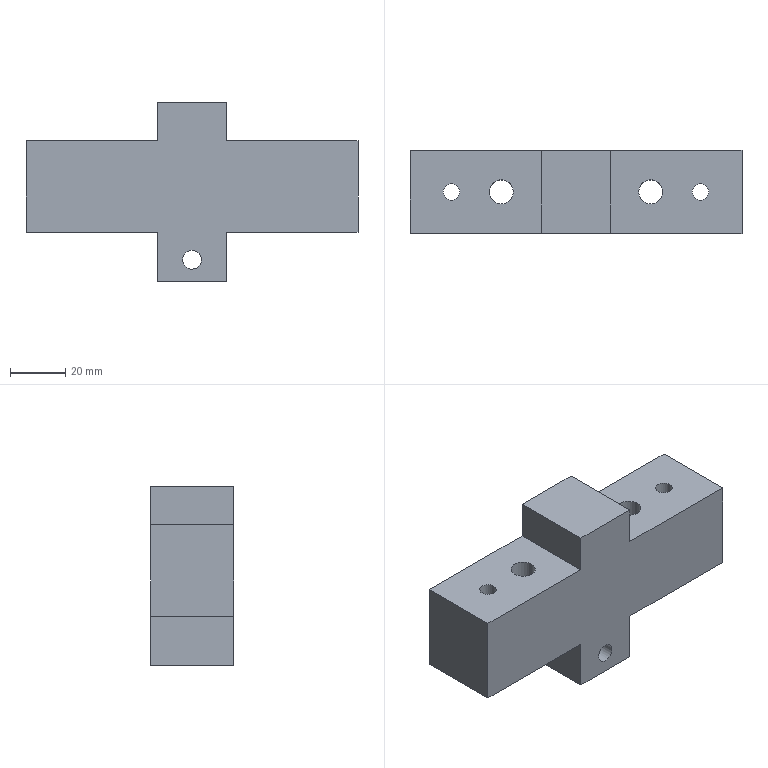Part | STEP file | 冲床-300配套压波_id542_x_t | 1 solid | 25 faces | box 120 x 30 x 65 mm | volume 132651 mm3 | plane 17 | cylinder 8 | commonest cylinder face diameters 10.7 x3 6 x2 8.7 x2 6.8 x1
STEP:
#1=CARTESIAN_POINT('',(1763.,85.,53.));
#2=VERTEX_POINT('',#1);
#3=CARTESIAN_POINT('',(1760.,85.,53.));
#4=DIRECTION('',(0.,0.,1.));
#5=DIRECTION('',(1.,0.,0.));
#6=AXIS2_PLACEMENT_3D('',#3,#4,#5);
#7=CIRCLE('',#6,3.);
#8=EDGE_CURVE('',#2,#2,#7,.T.);
#9=ORIENTED_EDGE('',*,*,#8,.F.);
#10=EDGE_LOOP('',(#9));
#11=FACE_BOUND('',#10,.T.);
#12=CARTESIAN_POINT('',(1745.,70.,53.));
#13=VERTEX_POINT('',#12);
#14=CARTESIAN_POINT('',(1792.5,70.,53.));
#15=VERTEX_POINT('',#14);
#16=CARTESIAN_POINT('',(1730.,70.,53.));
#17=DIRECTION('',(1.,0.,0.));
#18=VECTOR('',#17,1.);
#19=LINE('',#16,#18);
#20=EDGE_CURVE('',#13,#15,#19,.T.);
#21=ORIENTED_EDGE('',*,*,#20,.T.);
#22=CARTESIAN_POINT('',(1792.5,100.,53.));
#23=VERTEX_POINT('',#22);
#24=CARTESIAN_POINT('',(1792.5,100.,53.));
#25=DIRECTION('',(0.,-1.,0.));
#26=VECTOR('',#25,1.);
#27=LINE('',#24,#26);
#28=EDGE_CURVE('',#23,#15,#27,.T.);
#29=ORIENTED_EDGE('',*,*,#28,.F.);
#30=CARTESIAN_POINT('',(1745.,100.,53.));
#31=VERTEX_POINT('',#30);
#32=CARTESIAN_POINT('',(1730.,100.,53.));
#33=DIRECTION('',(1.,0.,0.));
#34=VECTOR('',#33,1.);
#35=LINE('',#32,#34);
#36=EDGE_CURVE('',#31,#23,#35,.T.);
#37=ORIENTED_EDGE('',*,*,#36,.F.);
#38=CARTESIAN_POINT('',(1745.,60.,53.));
#39=DIRECTION('',(0.,-1.,0.));
#40=VECTOR('',#39,1.);
#41=LINE('',#38,#40);
#42=EDGE_CURVE('',#31,#13,#41,.T.);
#43=ORIENTED_EDGE('',*,*,#42,.T.);
#44=EDGE_LOOP('',(#21,#29,#37,#43));
#45=FACE_BOUND('',#44,.T.);
#46=CARTESIAN_POINT('',(1782.35,85.,53.));
#47=VERTEX_POINT('',#46);
#48=CARTESIAN_POINT('',(1778.,85.,53.));
#49=DIRECTION('',(0.,0.,-1.));
#50=DIRECTION('',(1.,0.,0.));
#51=AXIS2_PLACEMENT_3D('',#48,#49,#50);
#52=CIRCLE('',#51,4.35);
#53=EDGE_CURVE('',#47,#47,#52,.T.);
#54=ORIENTED_EDGE('',*,*,#53,.T.);
#55=EDGE_LOOP('',(#54));
#56=FACE_BOUND('',#55,.T.);
#57=CARTESIAN_POINT('',(1730.,-80.,53.));
#58=DIRECTION('',(0.,0.,1.));
#59=DIRECTION('',(1.,0.,0.));
#60=AXIS2_PLACEMENT_3D('',#57,#58,#59);
#61=PLANE('',#60);
#62=ADVANCED_FACE('',(#11,#45,#56),#61,.T.);
#63=CARTESIAN_POINT('',(1827.65,85.,20.));
#64=VERTEX_POINT('',#63);
#65=CARTESIAN_POINT('',(1832.,85.,20.));
#66=DIRECTION('',(0.,0.,1.));
#67=DIRECTION('',(-1.,0.,0.));
#68=AXIS2_PLACEMENT_3D('',#65,#66,#67);
#69=CIRCLE('',#68,4.35);
#70=EDGE_CURVE('',#64,#64,#69,.T.);
#71=ORIENTED_EDGE('',*,*,#70,.T.);
#72=EDGE_LOOP('',(#71));
#73=FACE_BOUND('',#72,.T.);
#74=CARTESIAN_POINT('',(1855.35,85.,20.));
#75=VERTEX_POINT('',#74);
#76=CARTESIAN_POINT('',(1850.,85.,20.));
#77=DIRECTION('',(0.,0.,1.));
#78=DIRECTION('',(1.,0.,0.));
#79=AXIS2_PLACEMENT_3D('',#76,#77,#78);
#80=CIRCLE('',#79,5.35);
#81=EDGE_CURVE('',#75,#75,#80,.T.);
#82=ORIENTED_EDGE('',*,*,#81,.T.);
#83=EDGE_LOOP('',(#82));
#84=FACE_BOUND('',#83,.T.);
#85=CARTESIAN_POINT('',(1817.5,100.,20.));
#86=VERTEX_POINT('',#85);
#87=CARTESIAN_POINT('',(1817.5,70.,20.));
#88=VERTEX_POINT('',#87);
#89=CARTESIAN_POINT('',(1817.5,0.,20.));
#90=DIRECTION('',(0.,-1.,0.));
#91=VECTOR('',#90,1.);
#92=LINE('',#89,#91);
#93=EDGE_CURVE('',#86,#88,#92,.T.);
#94=ORIENTED_EDGE('',*,*,#93,.F.);
#95=CARTESIAN_POINT('',(1865.,100.,20.));
#96=VERTEX_POINT('',#95);
#97=CARTESIAN_POINT('',(1880.,100.,20.));
#98=DIRECTION('',(1.,0.,0.));
#99=VECTOR('',#98,1.);
#100=LINE('',#97,#99);
#101=EDGE_CURVE('',#86,#96,#100,.T.);
#102=ORIENTED_EDGE('',*,*,#101,.T.);
#103=CARTESIAN_POINT('',(1865.,70.,20.));
#104=VERTEX_POINT('',#103);
#105=CARTESIAN_POINT('',(1865.,-60.,20.));
#106=DIRECTION('',(0.,-1.,0.));
#107=VECTOR('',#106,1.);
#108=LINE('',#105,#107);
#109=EDGE_CURVE('',#96,#104,#108,.T.);
#110=ORIENTED_EDGE('',*,*,#109,.T.);
#111=CARTESIAN_POINT('',(1730.,70.,20.));
#112=DIRECTION('',(-1.,0.,0.));
#113=VECTOR('',#112,1.);
#114=LINE('',#111,#113);
#115=EDGE_CURVE('',#104,#88,#114,.T.);
#116=ORIENTED_EDGE('',*,*,#115,.T.);
#117=EDGE_LOOP('',(#94,#102,#110,#116));
#118=FACE_BOUND('',#117,.T.);
#119=CARTESIAN_POINT('',(1730.,-80.,20.));
#120=DIRECTION('',(0.,0.,-1.));
#121=DIRECTION('',(1.,0.,0.));
#122=AXIS2_PLACEMENT_3D('',#119,#120,#121);
#123=PLANE('',#122);
#124=ADVANCED_FACE('',(#73,#84,#118),#123,.T.);
#125=CARTESIAN_POINT('',(1805.,100.,15.35));
#126=VERTEX_POINT('',#125);
#127=CARTESIAN_POINT('',(1805.,100.,10.));
#128=DIRECTION('',(0.,-1.,0.));
#129=DIRECTION('',(0.,0.,1.));
#130=AXIS2_PLACEMENT_3D('',#127,#128,#129);
#131=CIRCLE('',#130,5.35);
#132=EDGE_CURVE('',#126,#126,#131,.T.);
#133=ORIENTED_EDGE('',*,*,#132,.T.);
#134=EDGE_LOOP('',(#133));
#135=FACE_BOUND('',#134,.T.);
#136=CARTESIAN_POINT('',(1792.5,100.,20.));
#137=VERTEX_POINT('',#136);
#138=CARTESIAN_POINT('',(1792.5,100.,2.));
#139=VERTEX_POINT('',#138);
#140=CARTESIAN_POINT('',(1792.5,100.,5.));
#141=DIRECTION('',(0.,0.,-1.));
#142=VECTOR('',#141,1.);
#143=LINE('',#140,#142);
#144=EDGE_CURVE('',#137,#139,#143,.T.);
#145=ORIENTED_EDGE('',*,*,#144,.F.);
#146=CARTESIAN_POINT('',(1745.,100.,20.));
#147=VERTEX_POINT('',#146);
#148=CARTESIAN_POINT('',(1880.,100.,20.));
#149=DIRECTION('',(1.,0.,0.));
#150=VECTOR('',#149,1.);
#151=LINE('',#148,#150);
#152=EDGE_CURVE('',#147,#137,#151,.T.);
#153=ORIENTED_EDGE('',*,*,#152,.F.);
#154=CARTESIAN_POINT('',(1745.,100.,145.));
#155=DIRECTION('',(0.,0.,-1.));
#156=VECTOR('',#155,1.);
#157=LINE('',#154,#156);
#158=EDGE_CURVE('',#31,#147,#157,.T.);
#159=ORIENTED_EDGE('',*,*,#158,.F.);
#160=ORIENTED_EDGE('',*,*,#36,.T.);
#161=CARTESIAN_POINT('',(1792.5,100.,67.));
#162=VERTEX_POINT('',#161);
#163=CARTESIAN_POINT('',(1792.5,100.,68.));
#164=DIRECTION('',(0.,0.,-1.));
#165=VECTOR('',#164,1.);
#166=LINE('',#163,#165);
#167=EDGE_CURVE('',#162,#23,#166,.T.);
#168=ORIENTED_EDGE('',*,*,#167,.F.);
#169=CARTESIAN_POINT('',(1817.5,100.,67.));
#170=VERTEX_POINT('',#169);
#171=CARTESIAN_POINT('',(1730.,100.,67.));
#172=DIRECTION('',(1.,0.,0.));
#173=VECTOR('',#172,1.);
#174=LINE('',#171,#173);
#175=EDGE_CURVE('',#162,#170,#174,.T.);
#176=ORIENTED_EDGE('',*,*,#175,.T.);
#177=CARTESIAN_POINT('',(1817.5,100.,53.));
#178=VERTEX_POINT('',#177);
#179=CARTESIAN_POINT('',(1817.5,100.,68.));
#180=DIRECTION('',(0.,0.,-1.));
#181=VECTOR('',#180,1.);
#182=LINE('',#179,#181);
#183=EDGE_CURVE('',#170,#178,#182,.T.);
#184=ORIENTED_EDGE('',*,*,#183,.T.);
#185=CARTESIAN_POINT('',(1865.,100.,53.));
#186=VERTEX_POINT('',#185);
#187=CARTESIAN_POINT('',(1730.,100.,53.));
#188=DIRECTION('',(1.,0.,0.));
#189=VECTOR('',#188,1.);
#190=LINE('',#187,#189);
#191=EDGE_CURVE('',#178,#186,#190,.T.);
#192=ORIENTED_EDGE('',*,*,#191,.T.);
#193=CARTESIAN_POINT('',(1865.,100.,150.));
#194=DIRECTION('',(0.,0.,-1.));
#195=VECTOR('',#194,1.);
#196=LINE('',#193,#195);
#197=EDGE_CURVE('',#186,#96,#196,.T.);
#198=ORIENTED_EDGE('',*,*,#197,.T.);
#199=ORIENTED_EDGE('',*,*,#101,.F.);
#200=CARTESIAN_POINT('',(1817.5,100.,2.));
#201=VERTEX_POINT('',#200);
#202=CARTESIAN_POINT('',(1817.5,100.,20.));
#203=DIRECTION('',(0.,0.,-1.));
#204=VECTOR('',#203,1.);
#205=LINE('',#202,#204);
#206=EDGE_CURVE('',#86,#201,#205,.T.);
#207=ORIENTED_EDGE('',*,*,#206,.T.);
#208=CARTESIAN_POINT('',(1730.,100.,2.));
#209=DIRECTION('',(-1.,0.,0.));
#210=VECTOR('',#209,1.);
#211=LINE('',#208,#210);
#212=EDGE_CURVE('',#201,#139,#211,.T.);
#213=ORIENTED_EDGE('',*,*,#212,.T.);
#214=EDGE_LOOP('',(#145,#153,#159,#160,#168,#176,#184,#192,#198,#199,#207,#213));
#215=FACE_BOUND('',#214,.T.);
#216=CARTESIAN_POINT('',(1880.,100.,150.));
#217=DIRECTION('',(0.,-1.,0.));
#218=DIRECTION('',(0.,0.,-1.));
#219=AXIS2_PLACEMENT_3D('',#216,#217,#218);
#220=PLANE('',#219);
#221=ADVANCED_FACE('',(#135,#215),#220,.F.);
#222=CARTESIAN_POINT('',(1855.35,85.,40.));
#223=VERTEX_POINT('',#222);
#224=CARTESIAN_POINT('',(1850.,85.,40.));
#225=DIRECTION('',(0.,0.,1.));
#226=DIRECTION('',(1.,0.,0.));
#227=AXIS2_PLACEMENT_3D('',#224,#225,#226);
#228=CIRCLE('',#227,5.35);
#229=EDGE_CURVE('',#223,#223,#228,.T.);
#230=ORIENTED_EDGE('',*,*,#229,.F.);
#231=EDGE_LOOP('',(#230));
#232=FACE_BOUND('',#231,.T.);
#233=CARTESIAN_POINT('',(1853.,85.,40.));
#234=VERTEX_POINT('',#233);
#235=CARTESIAN_POINT('',(1850.,85.,40.));
#236=DIRECTION('',(0.,0.,1.));
#237=DIRECTION('',(1.,0.,0.));
#238=AXIS2_PLACEMENT_3D('',#235,#236,#237);
#239=CIRCLE('',#238,3.);
#240=EDGE_CURVE('',#234,#234,#239,.T.);
#241=ORIENTED_EDGE('',*,*,#240,.T.);
#242=EDGE_LOOP('',(#241));
#243=FACE_BOUND('',#242,.T.);
#244=CARTESIAN_POINT('',(1850.,85.,40.));
#245=DIRECTION('',(0.,0.,-1.));
#246=DIRECTION('',(1.,0.,0.));
#247=AXIS2_PLACEMENT_3D('',#244,#245,#246);
#248=PLANE('',#247);
#249=ADVANCED_FACE('',(#232,#243),#248,.T.);
#250=CARTESIAN_POINT('',(1847.,85.,53.));
#251=VERTEX_POINT('',#250);
#252=CARTESIAN_POINT('',(1850.,85.,53.));
#253=DIRECTION('',(0.,0.,-1.));
#254=DIRECTION('',(-1.,0.,0.));
#255=AXIS2_PLACEMENT_3D('',#252,#253,#254);
#256=CIRCLE('',#255,3.);
#257=EDGE_CURVE('',#251,#251,#256,.T.);
#258=ORIENTED_EDGE('',*,*,#257,.F.);
#259=EDGE_LOOP('',(#258));
#260=FACE_BOUND('',#259,.T.);
#261=ORIENTED_EDGE('',*,*,#240,.F.);
#262=EDGE_LOOP('',(#261));
#263=FACE_BOUND('',#262,.T.);
#264=CARTESIAN_POINT('',(1850.,85.,-7.));
#265=DIRECTION('',(0.,0.,1.));
#266=DIRECTION('',(-1.,0.,0.));
#267=AXIS2_PLACEMENT_3D('',#264,#265,#266);
#268=CYLINDRICAL_SURFACE('',#267,3.);
#269=ADVANCED_FACE('',(#260,#263),#268,.F.);
#270=ORIENTED_EDGE('',*,*,#229,.T.);
#271=EDGE_LOOP('',(#270));
#272=FACE_BOUND('',#271,.T.);
#273=ORIENTED_EDGE('',*,*,#81,.F.);
#274=EDGE_LOOP('',(#273));
#275=FACE_BOUND('',#274,.T.);
#276=CARTESIAN_POINT('',(1850.,85.,40.));
#277=DIRECTION('',(0.,0.,-1.));
#278=DIRECTION('',(1.,0.,0.));
#279=AXIS2_PLACEMENT_3D('',#276,#277,#278);
#280=CYLINDRICAL_SURFACE('',#279,5.35);
#281=ADVANCED_FACE('',(#272,#275),#280,.F.);
#282=CARTESIAN_POINT('',(1754.65,85.,40.));
#283=VERTEX_POINT('',#282);
#284=CARTESIAN_POINT('',(1760.,85.,40.));
#285=DIRECTION('',(0.,0.,1.));
#286=DIRECTION('',(-1.,0.,0.));
#287=AXIS2_PLACEMENT_3D('',#284,#285,#286);
#288=CIRCLE('',#287,5.35);
#289=EDGE_CURVE('',#283,#283,#288,.T.);
#290=ORIENTED_EDGE('',*,*,#289,.F.);
#291=EDGE_LOOP('',(#290));
#292=FACE_BOUND('',#291,.T.);
#293=CARTESIAN_POINT('',(1757.,85.,40.));
#294=VERTEX_POINT('',#293);
#295=CARTESIAN_POINT('',(1760.,85.,40.));
#296=DIRECTION('',(0.,0.,1.));
#297=DIRECTION('',(-1.,0.,0.));
#298=AXIS2_PLACEMENT_3D('',#295,#296,#297);
#299=CIRCLE('',#298,3.);
#300=EDGE_CURVE('',#294,#294,#299,.T.);
#301=ORIENTED_EDGE('',*,*,#300,.T.);
#302=EDGE_LOOP('',(#301));
#303=FACE_BOUND('',#302,.T.);
#304=CARTESIAN_POINT('',(1760.,85.,40.));
#305=DIRECTION('',(0.,0.,-1.));
#306=DIRECTION('',(-1.,0.,0.));
#307=AXIS2_PLACEMENT_3D('',#304,#305,#306);
#308=PLANE('',#307);
#309=ADVANCED_FACE('',(#292,#303),#308,.T.);
#310=ORIENTED_EDGE('',*,*,#8,.T.);
#311=EDGE_LOOP('',(#310));
#312=FACE_BOUND('',#311,.T.);
#313=ORIENTED_EDGE('',*,*,#300,.F.);
#314=EDGE_LOOP('',(#313));
#315=FACE_BOUND('',#314,.T.);
#316=CARTESIAN_POINT('',(1760.,85.,-7.));
#317=DIRECTION('',(0.,0.,1.));
#318=DIRECTION('',(1.,0.,0.));
#319=AXIS2_PLACEMENT_3D('',#316,#317,#318);
#320=CYLINDRICAL_SURFACE('',#319,3.);
#321=ADVANCED_FACE('',(#312,#315),#320,.F.);
#322=ORIENTED_EDGE('',*,*,#289,.T.);
#323=EDGE_LOOP('',(#322));
#324=FACE_BOUND('',#323,.T.);
#325=CARTESIAN_POINT('',(1754.65,85.,20.));
#326=VERTEX_POINT('',#325);
#327=CARTESIAN_POINT('',(1760.,85.,20.));
#328=DIRECTION('',(0.,0.,-1.));
#329=DIRECTION('',(-1.,0.,0.));
#330=AXIS2_PLACEMENT_3D('',#327,#328,#329);
#331=CIRCLE('',#330,5.35);
#332=EDGE_CURVE('',#326,#326,#331,.T.);
#333=ORIENTED_EDGE('',*,*,#332,.T.);
#334=EDGE_LOOP('',(#333));
#335=FACE_BOUND('',#334,.T.);
#336=CARTESIAN_POINT('',(1760.,85.,40.));
#337=DIRECTION('',(0.,0.,-1.));
#338=DIRECTION('',(-1.,0.,0.));
#339=AXIS2_PLACEMENT_3D('',#336,#337,#338);
#340=CYLINDRICAL_SURFACE('',#339,5.35);
#341=ADVANCED_FACE('',(#324,#335),#340,.F.);
#342=CARTESIAN_POINT('',(1817.5,70.,67.));
#343=VERTEX_POINT('',#342);
#344=CARTESIAN_POINT('',(1817.5,-80.,67.));
#345=DIRECTION('',(0.,-1.,0.));
#346=VECTOR('',#345,1.);
#347=LINE('',#344,#346);
#348=EDGE_CURVE('',#170,#343,#347,.T.);
#349=ORIENTED_EDGE('',*,*,#348,.F.);
#350=ORIENTED_EDGE('',*,*,#175,.F.);
#351=CARTESIAN_POINT('',(1792.5,70.,67.));
#352=VERTEX_POINT('',#351);
#353=CARTESIAN_POINT('',(1792.5,-80.,67.));
#354=DIRECTION('',(0.,1.,0.));
#355=VECTOR('',#354,1.);
#356=LINE('',#353,#355);
#357=EDGE_CURVE('',#352,#162,#356,.T.);
#358=ORIENTED_EDGE('',*,*,#357,.F.);
#359=CARTESIAN_POINT('',(1730.,70.,67.));
#360=DIRECTION('',(-1.,0.,0.));
#361=VECTOR('',#360,1.);
#362=LINE('',#359,#361);
#363=EDGE_CURVE('',#343,#352,#362,.T.);
#364=ORIENTED_EDGE('',*,*,#363,.F.);
#365=EDGE_LOOP('',(#349,#350,#358,#364));
#366=FACE_OUTER_BOUND('',#365,.T.);
#367=CARTESIAN_POINT('',(1730.,-80.,67.));
#368=DIRECTION('',(0.,0.,1.));
#369=DIRECTION('',(1.,0.,0.));
#370=AXIS2_PLACEMENT_3D('',#367,#368,#369);
#371=PLANE('',#370);
#372=ADVANCED_FACE('',(#366),#371,.T.);
#373=ORIENTED_EDGE('',*,*,#42,.F.);
#374=ORIENTED_EDGE('',*,*,#158,.T.);
#375=CARTESIAN_POINT('',(1745.,70.,20.));
#376=VERTEX_POINT('',#375);
#377=CARTESIAN_POINT('',(1745.,60.,20.));
#378=DIRECTION('',(0.,1.,0.));
#379=VECTOR('',#378,1.);
#380=LINE('',#377,#379);
#381=EDGE_CURVE('',#376,#147,#380,.T.);
#382=ORIENTED_EDGE('',*,*,#381,.F.);
#383=CARTESIAN_POINT('',(1745.,70.,150.));
#384=DIRECTION('',(0.,0.,-1.));
#385=VECTOR('',#384,1.);
#386=LINE('',#383,#385);
#387=EDGE_CURVE('',#13,#376,#386,.T.);
#388=ORIENTED_EDGE('',*,*,#387,.F.);
#389=EDGE_LOOP('',(#373,#374,#382,#388));
#390=FACE_OUTER_BOUND('',#389,.T.);
#391=CARTESIAN_POINT('',(1745.,60.,145.));
#392=DIRECTION('',(-1.,0.,0.));
#393=DIRECTION('',(0.,0.,1.));
#394=AXIS2_PLACEMENT_3D('',#391,#392,#393);
#395=PLANE('',#394);
#396=ADVANCED_FACE('',(#390),#395,.T.);
#397=CARTESIAN_POINT('',(1773.65,85.,20.));
#398=VERTEX_POINT('',#397);
#399=CARTESIAN_POINT('',(1778.,85.,20.));
#400=DIRECTION('',(0.,0.,1.));
#401=DIRECTION('',(-1.,0.,0.));
#402=AXIS2_PLACEMENT_3D('',#399,#400,#401);
#403=CIRCLE('',#402,4.35);
#404=EDGE_CURVE('',#398,#398,#403,.T.);
#405=ORIENTED_EDGE('',*,*,#404,.T.);
#406=EDGE_LOOP('',(#405));
#407=FACE_BOUND('',#406,.T.);
#408=ORIENTED_EDGE('',*,*,#332,.F.);
#409=EDGE_LOOP('',(#408));
#410=FACE_BOUND('',#409,.T.);
#411=CARTESIAN_POINT('',(1792.5,70.,20.));
#412=VERTEX_POINT('',#411);
#413=CARTESIAN_POINT('',(1730.,70.,20.));
#414=DIRECTION('',(-1.,0.,0.));
#415=VECTOR('',#414,1.);
#416=LINE('',#413,#415);
#417=EDGE_CURVE('',#412,#376,#416,.T.);
#418=ORIENTED_EDGE('',*,*,#417,.T.);
#419=ORIENTED_EDGE('',*,*,#381,.T.);
#420=ORIENTED_EDGE('',*,*,#152,.T.);
#421=CARTESIAN_POINT('',(1792.5,0.,20.));
#422=DIRECTION('',(0.,1.,0.));
#423=VECTOR('',#422,1.);
#424=LINE('',#421,#423);
#425=EDGE_CURVE('',#412,#137,#424,.T.);
#426=ORIENTED_EDGE('',*,*,#425,.F.);
#427=EDGE_LOOP('',(#418,#419,#420,#426));
#428=FACE_BOUND('',#427,.T.);
#429=CARTESIAN_POINT('',(1730.,-80.,20.));
#430=DIRECTION('',(0.,0.,-1.));
#431=DIRECTION('',(1.,0.,0.));
#432=AXIS2_PLACEMENT_3D('',#429,#430,#431);
#433=PLANE('',#432);
#434=ADVANCED_FACE('',(#407,#410,#428),#433,.T.);
#435=CARTESIAN_POINT('',(1817.5,70.,2.));
#436=VERTEX_POINT('',#435);
#437=CARTESIAN_POINT('',(1817.5,-80.,2.));
#438=DIRECTION('',(0.,1.,0.));
#439=VECTOR('',#438,1.);
#440=LINE('',#437,#439);
#441=EDGE_CURVE('',#436,#201,#440,.T.);
#442=ORIENTED_EDGE('',*,*,#441,.F.);
#443=CARTESIAN_POINT('',(1792.5,70.,2.));
#444=VERTEX_POINT('',#443);
#445=CARTESIAN_POINT('',(1730.,70.,2.));
#446=DIRECTION('',(1.,0.,0.));
#447=VECTOR('',#446,1.);
#448=LINE('',#445,#447);
#449=EDGE_CURVE('',#444,#436,#448,.T.);
#450=ORIENTED_EDGE('',*,*,#449,.F.);
#451=CARTESIAN_POINT('',(1792.5,-80.,2.));
#452=DIRECTION('',(0.,-1.,0.));
#453=VECTOR('',#452,1.);
#454=LINE('',#451,#453);
#455=EDGE_CURVE('',#139,#444,#454,.T.);
#456=ORIENTED_EDGE('',*,*,#455,.F.);
#457=ORIENTED_EDGE('',*,*,#212,.F.);
#458=EDGE_LOOP('',(#442,#450,#456,#457));
#459=FACE_OUTER_BOUND('',#458,.T.);
#460=CARTESIAN_POINT('',(1730.,-80.,2.));
#461=DIRECTION('',(0.,0.,-1.));
#462=DIRECTION('',(1.,0.,0.));
#463=AXIS2_PLACEMENT_3D('',#460,#461,#462);
#464=PLANE('',#463);
#465=ADVANCED_FACE('',(#459),#464,.T.);
#466=CARTESIAN_POINT('',(1865.,70.,53.));
#467=VERTEX_POINT('',#466);
#468=CARTESIAN_POINT('',(1865.,-60.,53.));
#469=DIRECTION('',(0.,1.,0.));
#470=VECTOR('',#469,1.);
#471=LINE('',#468,#470);
#472=EDGE_CURVE('',#467,#186,#471,.T.);
#473=ORIENTED_EDGE('',*,*,#472,.F.);
#474=CARTESIAN_POINT('',(1865.,70.,145.));
#475=DIRECTION('',(0.,0.,-1.));
#476=VECTOR('',#475,1.);
#477=LINE('',#474,#476);
#478=EDGE_CURVE('',#467,#104,#477,.T.);
#479=ORIENTED_EDGE('',*,*,#478,.T.);
#480=ORIENTED_EDGE('',*,*,#109,.F.);
#481=ORIENTED_EDGE('',*,*,#197,.F.);
#482=EDGE_LOOP('',(#473,#479,#480,#481));
#483=FACE_OUTER_BOUND('',#482,.T.);
#484=CARTESIAN_POINT('',(1865.,-60.,145.));
#485=DIRECTION('',(1.,0.,0.));
#486=DIRECTION('',(0.,0.,-1.));
#487=AXIS2_PLACEMENT_3D('',#484,#485,#486);
#488=PLANE('',#487);
#489=ADVANCED_FACE('',(#483),#488,.T.);
#490=CARTESIAN_POINT('',(1808.4,70.,10.));
#491=VERTEX_POINT('',#490);
#492=CARTESIAN_POINT('',(1805.,70.,10.));
#493=DIRECTION('',(0.,1.,0.));
#494=DIRECTION('',(1.,0.,0.));
#495=AXIS2_PLACEMENT_3D('',#492,#493,#494);
#496=CIRCLE('',#495,3.4);
#497=EDGE_CURVE('',#491,#491,#496,.T.);
#498=ORIENTED_EDGE('',*,*,#497,.T.);
#499=EDGE_LOOP('',(#498));
#500=FACE_BOUND('',#499,.T.);
#501=ORIENTED_EDGE('',*,*,#363,.T.);
#502=CARTESIAN_POINT('',(1792.5,70.,150.));
#503=DIRECTION('',(0.,0.,-1.));
#504=VECTOR('',#503,1.);
#505=LINE('',#502,#504);
#506=EDGE_CURVE('',#352,#15,#505,.T.);
#507=ORIENTED_EDGE('',*,*,#506,.T.);
#508=ORIENTED_EDGE('',*,*,#20,.F.);
#509=ORIENTED_EDGE('',*,*,#387,.T.);
#510=ORIENTED_EDGE('',*,*,#417,.F.);
#511=CARTESIAN_POINT('',(1792.5,70.,150.));
#512=DIRECTION('',(0.,0.,-1.));
#513=VECTOR('',#512,1.);
#514=LINE('',#511,#513);
#515=EDGE_CURVE('',#412,#444,#514,.T.);
#516=ORIENTED_EDGE('',*,*,#515,.T.);
#517=ORIENTED_EDGE('',*,*,#449,.T.);
#518=CARTESIAN_POINT('',(1817.5,70.,150.));
#519=DIRECTION('',(0.,0.,1.));
#520=VECTOR('',#519,1.);
#521=LINE('',#518,#520);
#522=EDGE_CURVE('',#436,#88,#521,.T.);
#523=ORIENTED_EDGE('',*,*,#522,.T.);
#524=ORIENTED_EDGE('',*,*,#115,.F.);
#525=ORIENTED_EDGE('',*,*,#478,.F.);
#526=CARTESIAN_POINT('',(1817.5,70.,53.));
#527=VERTEX_POINT('',#526);
#528=CARTESIAN_POINT('',(1730.,70.,53.));
#529=DIRECTION('',(1.,0.,0.));
#530=VECTOR('',#529,1.);
#531=LINE('',#528,#530);
#532=EDGE_CURVE('',#527,#467,#531,.T.);
#533=ORIENTED_EDGE('',*,*,#532,.F.);
#534=CARTESIAN_POINT('',(1817.5,70.,150.));
#535=DIRECTION('',(0.,0.,1.));
#536=VECTOR('',#535,1.);
#537=LINE('',#534,#536);
#538=EDGE_CURVE('',#527,#343,#537,.T.);
#539=ORIENTED_EDGE('',*,*,#538,.T.);
#540=EDGE_LOOP('',(#501,#507,#508,#509,#510,#516,#517,#523,#524,#525,#533,#539));
#541=FACE_BOUND('',#540,.T.);
#542=CARTESIAN_POINT('',(1730.,70.,150.));
#543=DIRECTION('',(0.,1.,0.));
#544=DIRECTION('',(-1.,0.,0.));
#545=AXIS2_PLACEMENT_3D('',#542,#543,#544);
#546=PLANE('',#545);
#547=ADVANCED_FACE('',(#500,#541),#546,.F.);
#548=CARTESIAN_POINT('',(1836.35,85.,53.));
#549=VERTEX_POINT('',#548);
#550=CARTESIAN_POINT('',(1832.,85.,53.));
#551=DIRECTION('',(0.,0.,-1.));
#552=DIRECTION('',(1.,0.,0.));
#553=AXIS2_PLACEMENT_3D('',#550,#551,#552);
#554=CIRCLE('',#553,4.35);
#555=EDGE_CURVE('',#549,#549,#554,.T.);
#556=ORIENTED_EDGE('',*,*,#555,.T.);
#557=EDGE_LOOP('',(#556));
#558=FACE_BOUND('',#557,.T.);
#559=ORIENTED_EDGE('',*,*,#532,.T.);
#560=ORIENTED_EDGE('',*,*,#472,.T.);
#561=ORIENTED_EDGE('',*,*,#191,.F.);
#562=CARTESIAN_POINT('',(1817.5,58.462,53.));
#563=DIRECTION('',(0.,1.,0.));
#564=VECTOR('',#563,1.);
#565=LINE('',#562,#564);
#566=EDGE_CURVE('',#527,#178,#565,.T.);
#567=ORIENTED_EDGE('',*,*,#566,.F.);
#568=EDGE_LOOP('',(#559,#560,#561,#567));
#569=FACE_BOUND('',#568,.T.);
#570=ORIENTED_EDGE('',*,*,#257,.T.);
#571=EDGE_LOOP('',(#570));
#572=FACE_BOUND('',#571,.T.);
#573=CARTESIAN_POINT('',(1730.,-80.,53.));
#574=DIRECTION('',(0.,0.,1.));
#575=DIRECTION('',(1.,0.,0.));
#576=AXIS2_PLACEMENT_3D('',#573,#574,#575);
#577=PLANE('',#576);
#578=ADVANCED_FACE('',(#558,#569,#572),#577,.T.);
#579=ORIENTED_EDGE('',*,*,#357,.T.);
#580=ORIENTED_EDGE('',*,*,#167,.T.);
#581=ORIENTED_EDGE('',*,*,#28,.T.);
#582=ORIENTED_EDGE('',*,*,#506,.F.);
#583=EDGE_LOOP('',(#579,#580,#581,#582));
#584=FACE_OUTER_BOUND('',#583,.T.);
#585=CARTESIAN_POINT('',(1792.5,100.,68.));
#586=DIRECTION('',(1.,0.,0.));
#587=DIRECTION('',(0.,0.,-1.));
#588=AXIS2_PLACEMENT_3D('',#585,#586,#587);
#589=PLANE('',#588);
#590=ADVANCED_FACE('',(#584),#589,.F.);
#591=ORIENTED_EDGE('',*,*,#348,.T.);
#592=ORIENTED_EDGE('',*,*,#538,.F.);
#593=ORIENTED_EDGE('',*,*,#566,.T.);
#594=ORIENTED_EDGE('',*,*,#183,.F.);
#595=EDGE_LOOP('',(#591,#592,#593,#594));
#596=FACE_OUTER_BOUND('',#595,.T.);
#597=CARTESIAN_POINT('',(1817.5,58.462,68.));
#598=DIRECTION('',(-1.,0.,0.));
#599=DIRECTION('',(0.,0.,1.));
#600=AXIS2_PLACEMENT_3D('',#597,#598,#599);
#601=PLANE('',#600);
#602=ADVANCED_FACE('',(#596),#601,.F.);
#603=ORIENTED_EDGE('',*,*,#441,.T.);
#604=ORIENTED_EDGE('',*,*,#206,.F.);
#605=ORIENTED_EDGE('',*,*,#93,.T.);
#606=ORIENTED_EDGE('',*,*,#522,.F.);
#607=EDGE_LOOP('',(#603,#604,#605,#606));
#608=FACE_OUTER_BOUND('',#607,.T.);
#609=CARTESIAN_POINT('',(1817.5,58.462,5.));
#610=DIRECTION('',(-1.,0.,0.));
#611=DIRECTION('',(0.,0.,-1.));
#612=AXIS2_PLACEMENT_3D('',#609,#610,#611);
#613=PLANE('',#612);
#614=ADVANCED_FACE('',(#608),#613,.F.);
#615=ORIENTED_EDGE('',*,*,#455,.T.);
#616=ORIENTED_EDGE('',*,*,#515,.F.);
#617=ORIENTED_EDGE('',*,*,#425,.T.);
#618=ORIENTED_EDGE('',*,*,#144,.T.);
#619=EDGE_LOOP('',(#615,#616,#617,#618));
#620=FACE_OUTER_BOUND('',#619,.T.);
#621=CARTESIAN_POINT('',(1792.5,100.,5.));
#622=DIRECTION('',(1.,0.,0.));
#623=DIRECTION('',(0.,0.,1.));
#624=AXIS2_PLACEMENT_3D('',#621,#622,#623);
#625=PLANE('',#624);
#626=ADVANCED_FACE('',(#620),#625,.F.);
#627=ORIENTED_EDGE('',*,*,#404,.F.);
#628=EDGE_LOOP('',(#627));
#629=FACE_BOUND('',#628,.T.);
#630=ORIENTED_EDGE('',*,*,#53,.F.);
#631=EDGE_LOOP('',(#630));
#632=FACE_BOUND('',#631,.T.);
#633=CARTESIAN_POINT('',(1778.,85.,20.));
#634=DIRECTION('',(0.,0.,1.));
#635=DIRECTION('',(1.,0.,0.));
#636=AXIS2_PLACEMENT_3D('',#633,#634,#635);
#637=CYLINDRICAL_SURFACE('',#636,4.35);
#638=ADVANCED_FACE('',(#629,#632),#637,.F.);
#639=ORIENTED_EDGE('',*,*,#70,.F.);
#640=EDGE_LOOP('',(#639));
#641=FACE_BOUND('',#640,.T.);
#642=ORIENTED_EDGE('',*,*,#555,.F.);
#643=EDGE_LOOP('',(#642));
#644=FACE_BOUND('',#643,.T.);
#645=CARTESIAN_POINT('',(1832.,85.,-49.));
#646=DIRECTION('',(0.,0.,1.));
#647=DIRECTION('',(1.,0.,0.));
#648=AXIS2_PLACEMENT_3D('',#645,#646,#647);
#649=CYLINDRICAL_SURFACE('',#648,4.35);
#650=ADVANCED_FACE('',(#641,#644),#649,.F.);
#651=CARTESIAN_POINT('',(1805.,85.,13.4));
#652=VERTEX_POINT('',#651);
#653=CARTESIAN_POINT('',(1805.,85.,10.));
#654=DIRECTION('',(0.,1.,0.));
#655=DIRECTION('',(0.,0.,1.));
#656=AXIS2_PLACEMENT_3D('',#653,#654,#655);
#657=CIRCLE('',#656,3.4);
#658=EDGE_CURVE('',#652,#652,#657,.T.);
#659=ORIENTED_EDGE('',*,*,#658,.T.);
#660=EDGE_LOOP('',(#659));
#661=FACE_BOUND('',#660,.T.);
#662=ORIENTED_EDGE('',*,*,#497,.F.);
#663=EDGE_LOOP('',(#662));
#664=FACE_BOUND('',#663,.T.);
#665=CARTESIAN_POINT('',(1805.,12.157,10.));
#666=DIRECTION('',(0.,-1.,0.));
#667=DIRECTION('',(0.,0.,1.));
#668=AXIS2_PLACEMENT_3D('',#665,#666,#667);
#669=CYLINDRICAL_SURFACE('',#668,3.4);
#670=ADVANCED_FACE('',(#661,#664),#669,.F.);
#671=ORIENTED_EDGE('',*,*,#658,.F.);
#672=EDGE_LOOP('',(#671));
#673=FACE_BOUND('',#672,.T.);
#674=CARTESIAN_POINT('',(1805.,85.,15.35));
#675=VERTEX_POINT('',#674);
#676=CARTESIAN_POINT('',(1805.,85.,10.));
#677=DIRECTION('',(0.,1.,0.));
#678=DIRECTION('',(0.,0.,1.));
#679=AXIS2_PLACEMENT_3D('',#676,#677,#678);
#680=CIRCLE('',#679,5.35);
#681=EDGE_CURVE('',#675,#675,#680,.T.);
#682=ORIENTED_EDGE('',*,*,#681,.T.);
#683=EDGE_LOOP('',(#682));
#684=FACE_BOUND('',#683,.T.);
#685=CARTESIAN_POINT('',(1805.,85.,10.));
#686=DIRECTION('',(0.,-1.,0.));
#687=DIRECTION('',(0.,0.,1.));
#688=AXIS2_PLACEMENT_3D('',#685,#686,#687);
#689=PLANE('',#688);
#690=ADVANCED_FACE('',(#673,#684),#689,.F.);
#691=ORIENTED_EDGE('',*,*,#681,.F.);
#692=EDGE_LOOP('',(#691));
#693=FACE_BOUND('',#692,.T.);
#694=ORIENTED_EDGE('',*,*,#132,.F.);
#695=EDGE_LOOP('',(#694));
#696=FACE_BOUND('',#695,.T.);
#697=CARTESIAN_POINT('',(1805.,100.,10.));
#698=DIRECTION('',(0.,-1.,0.));
#699=DIRECTION('',(0.,0.,1.));
#700=AXIS2_PLACEMENT_3D('',#697,#698,#699);
#701=CYLINDRICAL_SURFACE('',#700,5.35);
#702=ADVANCED_FACE('',(#693,#696),#701,.F.);
#703=CLOSED_SHELL('',(#62,#124,#221,#249,#269,#281,#309,#321,#341,#372,#396,#434,#465,#489,#547,#578,#590,#602,#614,#626,#638,#650,#670,#690,#702));
#704=MANIFOLD_SOLID_BREP('',#703);
#705=(LENGTH_UNIT()NAMED_UNIT(*)SI_UNIT(.MILLI.,.METRE.));
#706=UNCERTAINTY_MEASURE_WITH_UNIT(LENGTH_MEASURE(0.00002),#705,'','');
#707=(NAMED_UNIT(*)PLANE_ANGLE_UNIT()SI_UNIT($,.RADIAN.));
#708=PLANE_ANGLE_MEASURE_WITH_UNIT(PLANE_ANGLE_MEASURE(0.01745),#707);
#709=DIMENSIONAL_EXPONENTS(0.,0.,0.,0.,0.,0.,0.);
#710=(CONVERSION_BASED_UNIT('DEGREE',#708)NAMED_UNIT(#709)PLANE_ANGLE_UNIT());
#711=(NAMED_UNIT(*)SI_UNIT($,.STERADIAN.)SOLID_ANGLE_UNIT());
#712=(GEOMETRIC_REPRESENTATION_CONTEXT(3)GLOBAL_UNCERTAINTY_ASSIGNED_CONTEXT((#706))GLOBAL_UNIT_ASSIGNED_CONTEXT((#705,#710,#711))REPRESENTATION_CONTEXT('',''));
#713=ADVANCED_BREP_SHAPE_REPRESENTATION('',(#704),#712);